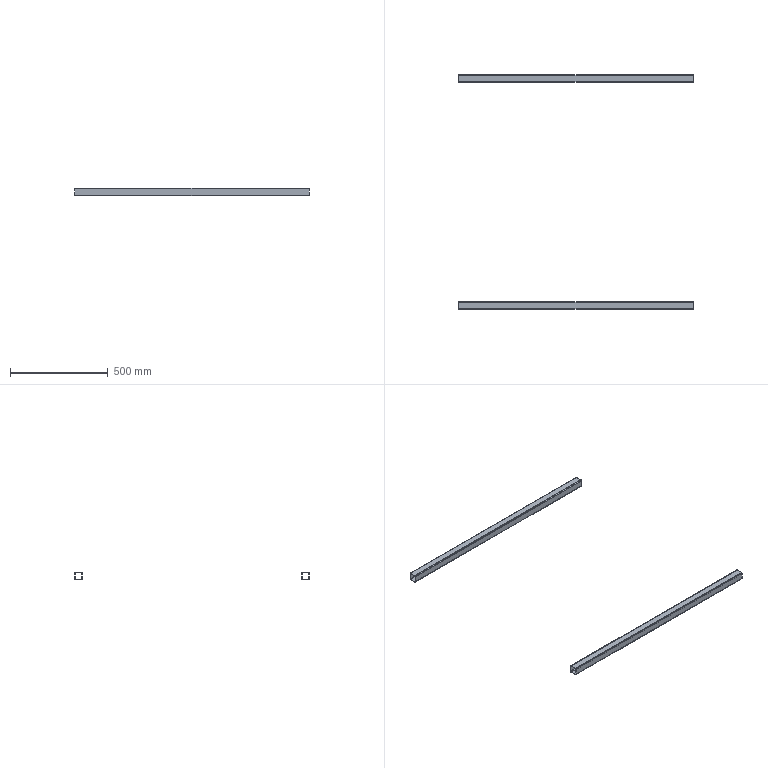Part | SolidWorks | features WeldMemberFeat 1, WeldmentFeature 1 | 2 solids | 36 faces | box 1200 x 1200 x 40 mm | volume 799721 mm3 | plane 20 | cylinder 16 | commonest cylinder face diameters 4.6 x8 9.2 x8
STEP:
#1=CARTESIAN_POINT('',(0.,20.,15.4));
#2=VERTEX_POINT('',#1);
#3=CARTESIAN_POINT('',(0.,15.4,20.));
#4=VERTEX_POINT('',#3);
#5=CARTESIAN_POINT('',(0.,15.4,15.4));
#6=DIRECTION('',(1.,0.,0.));
#7=DIRECTION('',(0.,0.,-1.));
#8=AXIS2_PLACEMENT_3D('',#5,#6,#7);
#9=CIRCLE('',#8,4.6);
#10=EDGE_CURVE('',#2,#4,#9,.T.);
#11=ORIENTED_EDGE('',*,*,#10,.T.);
#12=CARTESIAN_POINT('',(1200.,15.4,20.));
#13=VERTEX_POINT('',#12);
#14=CARTESIAN_POINT('',(1200.,15.4,20.));
#15=DIRECTION('',(-1.,0.,0.));
#16=VECTOR('',#15,1000.);
#17=LINE('',#14,#16);
#18=EDGE_CURVE('',#13,#4,#17,.T.);
#19=ORIENTED_EDGE('',*,*,#18,.F.);
#20=CARTESIAN_POINT('',(1200.,20.,15.4));
#21=VERTEX_POINT('',#20);
#22=CARTESIAN_POINT('',(1200.,15.4,15.4));
#23=DIRECTION('',(1.,0.,0.));
#24=DIRECTION('',(0.,0.,-1.));
#25=AXIS2_PLACEMENT_3D('',#22,#23,#24);
#26=CIRCLE('',#25,4.6);
#27=EDGE_CURVE('',#21,#13,#26,.T.);
#28=ORIENTED_EDGE('',*,*,#27,.F.);
#29=CARTESIAN_POINT('',(1200.,20.,15.4));
#30=DIRECTION('',(-1.,0.,0.));
#31=VECTOR('',#30,1000.);
#32=LINE('',#29,#31);
#33=EDGE_CURVE('',#21,#2,#32,.T.);
#34=ORIENTED_EDGE('',*,*,#33,.T.);
#35=EDGE_LOOP('',(#11,#19,#28,#34));
#36=FACE_OUTER_BOUND('',#35,.T.);
#37=CARTESIAN_POINT('',(1200.,15.4,15.4));
#38=DIRECTION('',(-1.,0.,0.));
#39=DIRECTION('',(0.,0.,1.));
#40=AXIS2_PLACEMENT_3D('',#37,#38,#39);
#41=CYLINDRICAL_SURFACE('',#40,4.6);
#42=ADVANCED_FACE('',(#36),#41,.T.);
#43=CARTESIAN_POINT('',(0.,-15.4,20.));
#44=VERTEX_POINT('',#43);
#45=CARTESIAN_POINT('',(0.,15.4,20.));
#46=DIRECTION('',(0.,-1.,0.));
#47=VECTOR('',#46,1000.);
#48=LINE('',#45,#47);
#49=EDGE_CURVE('',#4,#44,#48,.T.);
#50=ORIENTED_EDGE('',*,*,#49,.T.);
#51=CARTESIAN_POINT('',(1200.,-15.4,20.));
#52=VERTEX_POINT('',#51);
#53=CARTESIAN_POINT('',(1200.,-15.4,20.));
#54=DIRECTION('',(-1.,0.,0.));
#55=VECTOR('',#54,1000.);
#56=LINE('',#53,#55);
#57=EDGE_CURVE('',#52,#44,#56,.T.);
#58=ORIENTED_EDGE('',*,*,#57,.F.);
#59=CARTESIAN_POINT('',(1200.,15.4,20.));
#60=DIRECTION('',(0.,-1.,0.));
#61=VECTOR('',#60,1000.);
#62=LINE('',#59,#61);
#63=EDGE_CURVE('',#13,#52,#62,.T.);
#64=ORIENTED_EDGE('',*,*,#63,.F.);
#65=ORIENTED_EDGE('',*,*,#18,.T.);
#66=EDGE_LOOP('',(#50,#58,#64,#65));
#67=FACE_OUTER_BOUND('',#66,.T.);
#68=CARTESIAN_POINT('',(1200.,15.4,20.));
#69=DIRECTION('',(0.,0.,-1.));
#70=DIRECTION('',(0.,1.,0.));
#71=AXIS2_PLACEMENT_3D('',#68,#69,#70);
#72=PLANE('',#71);
#73=ADVANCED_FACE('',(#67),#72,.F.);
#74=CARTESIAN_POINT('',(0.,-20.,15.4));
#75=VERTEX_POINT('',#74);
#76=CARTESIAN_POINT('',(0.,-15.4,15.4));
#77=DIRECTION('',(1.,0.,0.));
#78=DIRECTION('',(0.,0.,-1.));
#79=AXIS2_PLACEMENT_3D('',#76,#77,#78);
#80=CIRCLE('',#79,4.6);
#81=EDGE_CURVE('',#44,#75,#80,.T.);
#82=ORIENTED_EDGE('',*,*,#81,.T.);
#83=CARTESIAN_POINT('',(1200.,-20.,15.4));
#84=VERTEX_POINT('',#83);
#85=CARTESIAN_POINT('',(1200.,-20.,15.4));
#86=DIRECTION('',(-1.,0.,0.));
#87=VECTOR('',#86,1000.);
#88=LINE('',#85,#87);
#89=EDGE_CURVE('',#84,#75,#88,.T.);
#90=ORIENTED_EDGE('',*,*,#89,.F.);
#91=CARTESIAN_POINT('',(1200.,-15.4,15.4));
#92=DIRECTION('',(1.,0.,0.));
#93=DIRECTION('',(0.,0.,-1.));
#94=AXIS2_PLACEMENT_3D('',#91,#92,#93);
#95=CIRCLE('',#94,4.6);
#96=EDGE_CURVE('',#52,#84,#95,.T.);
#97=ORIENTED_EDGE('',*,*,#96,.F.);
#98=ORIENTED_EDGE('',*,*,#57,.T.);
#99=EDGE_LOOP('',(#82,#90,#97,#98));
#100=FACE_OUTER_BOUND('',#99,.T.);
#101=CARTESIAN_POINT('',(1200.,-15.4,15.4));
#102=DIRECTION('',(-1.,0.,0.));
#103=DIRECTION('',(0.,0.,1.));
#104=AXIS2_PLACEMENT_3D('',#101,#102,#103);
#105=CYLINDRICAL_SURFACE('',#104,4.6);
#106=ADVANCED_FACE('',(#100),#105,.T.);
#107=CARTESIAN_POINT('',(0.,-20.,-15.4));
#108=VERTEX_POINT('',#107);
#109=CARTESIAN_POINT('',(0.,-20.,-15.4));
#110=DIRECTION('',(0.,0.,-1.));
#111=VECTOR('',#110,1000.);
#112=LINE('',#109,#111);
#113=EDGE_CURVE('',#75,#108,#112,.T.);
#114=ORIENTED_EDGE('',*,*,#113,.T.);
#115=CARTESIAN_POINT('',(1200.,-20.,-15.4));
#116=VERTEX_POINT('',#115);
#117=CARTESIAN_POINT('',(1200.,-20.,-15.4));
#118=DIRECTION('',(-1.,0.,0.));
#119=VECTOR('',#118,1000.);
#120=LINE('',#117,#119);
#121=EDGE_CURVE('',#116,#108,#120,.T.);
#122=ORIENTED_EDGE('',*,*,#121,.F.);
#123=CARTESIAN_POINT('',(1200.,-20.,-15.4));
#124=DIRECTION('',(0.,0.,-1.));
#125=VECTOR('',#124,1000.);
#126=LINE('',#123,#125);
#127=EDGE_CURVE('',#84,#116,#126,.T.);
#128=ORIENTED_EDGE('',*,*,#127,.F.);
#129=ORIENTED_EDGE('',*,*,#89,.T.);
#130=EDGE_LOOP('',(#114,#122,#128,#129));
#131=FACE_OUTER_BOUND('',#130,.T.);
#132=CARTESIAN_POINT('',(1200.,-20.,-15.4));
#133=DIRECTION('',(0.,1.,0.));
#134=DIRECTION('',(0.,0.,1.));
#135=AXIS2_PLACEMENT_3D('',#132,#133,#134);
#136=PLANE('',#135);
#137=ADVANCED_FACE('',(#131),#136,.F.);
#138=CARTESIAN_POINT('',(0.,-15.4,-20.));
#139=VERTEX_POINT('',#138);
#140=CARTESIAN_POINT('',(0.,-15.4,-15.4));
#141=DIRECTION('',(1.,0.,0.));
#142=DIRECTION('',(0.,0.,-1.));
#143=AXIS2_PLACEMENT_3D('',#140,#141,#142);
#144=CIRCLE('',#143,4.6);
#145=EDGE_CURVE('',#108,#139,#144,.T.);
#146=ORIENTED_EDGE('',*,*,#145,.T.);
#147=CARTESIAN_POINT('',(1200.,-15.4,-20.));
#148=VERTEX_POINT('',#147);
#149=CARTESIAN_POINT('',(1200.,-15.4,-20.));
#150=DIRECTION('',(-1.,0.,0.));
#151=VECTOR('',#150,1000.);
#152=LINE('',#149,#151);
#153=EDGE_CURVE('',#148,#139,#152,.T.);
#154=ORIENTED_EDGE('',*,*,#153,.F.);
#155=CARTESIAN_POINT('',(1200.,-15.4,-15.4));
#156=DIRECTION('',(1.,0.,0.));
#157=DIRECTION('',(0.,0.,-1.));
#158=AXIS2_PLACEMENT_3D('',#155,#156,#157);
#159=CIRCLE('',#158,4.6);
#160=EDGE_CURVE('',#116,#148,#159,.T.);
#161=ORIENTED_EDGE('',*,*,#160,.F.);
#162=ORIENTED_EDGE('',*,*,#121,.T.);
#163=EDGE_LOOP('',(#146,#154,#161,#162));
#164=FACE_OUTER_BOUND('',#163,.T.);
#165=CARTESIAN_POINT('',(1200.,-15.4,-15.4));
#166=DIRECTION('',(-1.,0.,0.));
#167=DIRECTION('',(0.,0.,1.));
#168=AXIS2_PLACEMENT_3D('',#165,#166,#167);
#169=CYLINDRICAL_SURFACE('',#168,4.6);
#170=ADVANCED_FACE('',(#164),#169,.T.);
#171=CARTESIAN_POINT('',(0.,15.4,-20.));
#172=VERTEX_POINT('',#171);
#173=CARTESIAN_POINT('',(0.,-15.4,-20.));
#174=DIRECTION('',(0.,1.,0.));
#175=VECTOR('',#174,1000.);
#176=LINE('',#173,#175);
#177=EDGE_CURVE('',#139,#172,#176,.T.);
#178=ORIENTED_EDGE('',*,*,#177,.T.);
#179=CARTESIAN_POINT('',(1200.,15.4,-20.));
#180=VERTEX_POINT('',#179);
#181=CARTESIAN_POINT('',(1200.,15.4,-20.));
#182=DIRECTION('',(-1.,0.,0.));
#183=VECTOR('',#182,1000.);
#184=LINE('',#181,#183);
#185=EDGE_CURVE('',#180,#172,#184,.T.);
#186=ORIENTED_EDGE('',*,*,#185,.F.);
#187=CARTESIAN_POINT('',(1200.,-15.4,-20.));
#188=DIRECTION('',(0.,1.,0.));
#189=VECTOR('',#188,1000.);
#190=LINE('',#187,#189);
#191=EDGE_CURVE('',#148,#180,#190,.T.);
#192=ORIENTED_EDGE('',*,*,#191,.F.);
#193=ORIENTED_EDGE('',*,*,#153,.T.);
#194=EDGE_LOOP('',(#178,#186,#192,#193));
#195=FACE_OUTER_BOUND('',#194,.T.);
#196=CARTESIAN_POINT('',(1200.,-15.4,-20.));
#197=DIRECTION('',(0.,0.,1.));
#198=DIRECTION('',(0.,-1.,0.));
#199=AXIS2_PLACEMENT_3D('',#196,#197,#198);
#200=PLANE('',#199);
#201=ADVANCED_FACE('',(#195),#200,.F.);
#202=CARTESIAN_POINT('',(0.,20.,-15.4));
#203=VERTEX_POINT('',#202);
#204=CARTESIAN_POINT('',(0.,15.4,-15.4));
#205=DIRECTION('',(1.,0.,0.));
#206=DIRECTION('',(0.,0.,-1.));
#207=AXIS2_PLACEMENT_3D('',#204,#205,#206);
#208=CIRCLE('',#207,4.6);
#209=EDGE_CURVE('',#172,#203,#208,.T.);
#210=ORIENTED_EDGE('',*,*,#209,.T.);
#211=CARTESIAN_POINT('',(1200.,20.,-15.4));
#212=VERTEX_POINT('',#211);
#213=CARTESIAN_POINT('',(1200.,20.,-15.4));
#214=DIRECTION('',(-1.,0.,0.));
#215=VECTOR('',#214,1000.);
#216=LINE('',#213,#215);
#217=EDGE_CURVE('',#212,#203,#216,.T.);
#218=ORIENTED_EDGE('',*,*,#217,.F.);
#219=CARTESIAN_POINT('',(1200.,15.4,-15.4));
#220=DIRECTION('',(1.,0.,0.));
#221=DIRECTION('',(0.,0.,-1.));
#222=AXIS2_PLACEMENT_3D('',#219,#220,#221);
#223=CIRCLE('',#222,4.6);
#224=EDGE_CURVE('',#180,#212,#223,.T.);
#225=ORIENTED_EDGE('',*,*,#224,.F.);
#226=ORIENTED_EDGE('',*,*,#185,.T.);
#227=EDGE_LOOP('',(#210,#218,#225,#226));
#228=FACE_OUTER_BOUND('',#227,.T.);
#229=CARTESIAN_POINT('',(1200.,15.4,-15.4));
#230=DIRECTION('',(-1.,0.,0.));
#231=DIRECTION('',(0.,0.,1.));
#232=AXIS2_PLACEMENT_3D('',#229,#230,#231);
#233=CYLINDRICAL_SURFACE('',#232,4.6);
#234=ADVANCED_FACE('',(#228),#233,.T.);
#235=CARTESIAN_POINT('',(0.,-15.4,17.7));
#236=VERTEX_POINT('',#235);
#237=CARTESIAN_POINT('',(0.,-17.7,15.4));
#238=VERTEX_POINT('',#237);
#239=CARTESIAN_POINT('',(0.,-15.4,15.4));
#240=DIRECTION('',(1.,0.,0.));
#241=DIRECTION('',(0.,0.,-1.));
#242=AXIS2_PLACEMENT_3D('',#239,#240,#241);
#243=CIRCLE('',#242,2.3);
#244=EDGE_CURVE('',#236,#238,#243,.T.);
#245=ORIENTED_EDGE('',*,*,#244,.F.);
#246=CARTESIAN_POINT('',(1200.,-15.4,17.7));
#247=VERTEX_POINT('',#246);
#248=CARTESIAN_POINT('',(1200.,-15.4,17.7));
#249=DIRECTION('',(-1.,0.,0.));
#250=VECTOR('',#249,1000.);
#251=LINE('',#248,#250);
#252=EDGE_CURVE('',#247,#236,#251,.T.);
#253=ORIENTED_EDGE('',*,*,#252,.F.);
#254=CARTESIAN_POINT('',(1200.,-17.7,15.4));
#255=VERTEX_POINT('',#254);
#256=CARTESIAN_POINT('',(1200.,-15.4,15.4));
#257=DIRECTION('',(1.,0.,0.));
#258=DIRECTION('',(0.,0.,-1.));
#259=AXIS2_PLACEMENT_3D('',#256,#257,#258);
#260=CIRCLE('',#259,2.3);
#261=EDGE_CURVE('',#247,#255,#260,.T.);
#262=ORIENTED_EDGE('',*,*,#261,.T.);
#263=CARTESIAN_POINT('',(1200.,-17.7,15.4));
#264=DIRECTION('',(-1.,0.,0.));
#265=VECTOR('',#264,1000.);
#266=LINE('',#263,#265);
#267=EDGE_CURVE('',#255,#238,#266,.T.);
#268=ORIENTED_EDGE('',*,*,#267,.T.);
#269=EDGE_LOOP('',(#245,#253,#262,#268));
#270=FACE_OUTER_BOUND('',#269,.T.);
#271=CARTESIAN_POINT('',(1200.,-15.4,15.4));
#272=DIRECTION('',(-1.,0.,0.));
#273=DIRECTION('',(0.,0.,1.));
#274=AXIS2_PLACEMENT_3D('',#271,#272,#273);
#275=CYLINDRICAL_SURFACE('',#274,2.3);
#276=ADVANCED_FACE('',(#270),#275,.F.);
#277=CARTESIAN_POINT('',(0.,15.4,17.7));
#278=VERTEX_POINT('',#277);
#279=CARTESIAN_POINT('',(0.,15.4,17.7));
#280=DIRECTION('',(0.,-1.,0.));
#281=VECTOR('',#280,1000.);
#282=LINE('',#279,#281);
#283=EDGE_CURVE('',#278,#236,#282,.T.);
#284=ORIENTED_EDGE('',*,*,#283,.F.);
#285=CARTESIAN_POINT('',(1200.,15.4,17.7));
#286=VERTEX_POINT('',#285);
#287=CARTESIAN_POINT('',(1200.,15.4,17.7));
#288=DIRECTION('',(-1.,0.,0.));
#289=VECTOR('',#288,1000.);
#290=LINE('',#287,#289);
#291=EDGE_CURVE('',#286,#278,#290,.T.);
#292=ORIENTED_EDGE('',*,*,#291,.F.);
#293=CARTESIAN_POINT('',(1200.,15.4,17.7));
#294=DIRECTION('',(0.,-1.,0.));
#295=VECTOR('',#294,1000.);
#296=LINE('',#293,#295);
#297=EDGE_CURVE('',#286,#247,#296,.T.);
#298=ORIENTED_EDGE('',*,*,#297,.T.);
#299=ORIENTED_EDGE('',*,*,#252,.T.);
#300=EDGE_LOOP('',(#284,#292,#298,#299));
#301=FACE_OUTER_BOUND('',#300,.T.);
#302=CARTESIAN_POINT('',(1200.,15.4,17.7));
#303=DIRECTION('',(0.,0.,-1.));
#304=DIRECTION('',(0.,1.,0.));
#305=AXIS2_PLACEMENT_3D('',#302,#303,#304);
#306=PLANE('',#305);
#307=ADVANCED_FACE('',(#301),#306,.T.);
#308=CARTESIAN_POINT('',(0.,17.7,15.4));
#309=VERTEX_POINT('',#308);
#310=CARTESIAN_POINT('',(0.,15.4,15.4));
#311=DIRECTION('',(1.,0.,0.));
#312=DIRECTION('',(0.,0.,-1.));
#313=AXIS2_PLACEMENT_3D('',#310,#311,#312);
#314=CIRCLE('',#313,2.3);
#315=EDGE_CURVE('',#309,#278,#314,.T.);
#316=ORIENTED_EDGE('',*,*,#315,.F.);
#317=CARTESIAN_POINT('',(1200.,17.7,15.4));
#318=VERTEX_POINT('',#317);
#319=CARTESIAN_POINT('',(1200.,17.7,15.4));
#320=DIRECTION('',(-1.,0.,0.));
#321=VECTOR('',#320,1000.);
#322=LINE('',#319,#321);
#323=EDGE_CURVE('',#318,#309,#322,.T.);
#324=ORIENTED_EDGE('',*,*,#323,.F.);
#325=CARTESIAN_POINT('',(1200.,15.4,15.4));
#326=DIRECTION('',(1.,0.,0.));
#327=DIRECTION('',(0.,0.,-1.));
#328=AXIS2_PLACEMENT_3D('',#325,#326,#327);
#329=CIRCLE('',#328,2.3);
#330=EDGE_CURVE('',#318,#286,#329,.T.);
#331=ORIENTED_EDGE('',*,*,#330,.T.);
#332=ORIENTED_EDGE('',*,*,#291,.T.);
#333=EDGE_LOOP('',(#316,#324,#331,#332));
#334=FACE_OUTER_BOUND('',#333,.T.);
#335=CARTESIAN_POINT('',(1200.,15.4,15.4));
#336=DIRECTION('',(-1.,0.,0.));
#337=DIRECTION('',(0.,0.,1.));
#338=AXIS2_PLACEMENT_3D('',#335,#336,#337);
#339=CYLINDRICAL_SURFACE('',#338,2.3);
#340=ADVANCED_FACE('',(#334),#339,.F.);
#341=CARTESIAN_POINT('',(0.,17.7,-15.4));
#342=VERTEX_POINT('',#341);
#343=CARTESIAN_POINT('',(0.,17.7,15.4));
#344=DIRECTION('',(0.,0.,1.));
#345=VECTOR('',#344,1000.);
#346=LINE('',#343,#345);
#347=EDGE_CURVE('',#342,#309,#346,.T.);
#348=ORIENTED_EDGE('',*,*,#347,.F.);
#349=CARTESIAN_POINT('',(1200.,17.7,-15.4));
#350=VERTEX_POINT('',#349);
#351=CARTESIAN_POINT('',(1200.,17.7,-15.4));
#352=DIRECTION('',(-1.,0.,0.));
#353=VECTOR('',#352,1000.);
#354=LINE('',#351,#353);
#355=EDGE_CURVE('',#350,#342,#354,.T.);
#356=ORIENTED_EDGE('',*,*,#355,.F.);
#357=CARTESIAN_POINT('',(1200.,17.7,15.4));
#358=DIRECTION('',(0.,0.,1.));
#359=VECTOR('',#358,1000.);
#360=LINE('',#357,#359);
#361=EDGE_CURVE('',#350,#318,#360,.T.);
#362=ORIENTED_EDGE('',*,*,#361,.T.);
#363=ORIENTED_EDGE('',*,*,#323,.T.);
#364=EDGE_LOOP('',(#348,#356,#362,#363));
#365=FACE_OUTER_BOUND('',#364,.T.);
#366=CARTESIAN_POINT('',(1200.,17.7,15.4));
#367=DIRECTION('',(0.,-1.,0.));
#368=DIRECTION('',(0.,0.,-1.));
#369=AXIS2_PLACEMENT_3D('',#366,#367,#368);
#370=PLANE('',#369);
#371=ADVANCED_FACE('',(#365),#370,.T.);
#372=CARTESIAN_POINT('',(0.,15.4,-17.7));
#373=VERTEX_POINT('',#372);
#374=CARTESIAN_POINT('',(0.,15.4,-15.4));
#375=DIRECTION('',(1.,0.,0.));
#376=DIRECTION('',(0.,0.,-1.));
#377=AXIS2_PLACEMENT_3D('',#374,#375,#376);
#378=CIRCLE('',#377,2.3);
#379=EDGE_CURVE('',#373,#342,#378,.T.);
#380=ORIENTED_EDGE('',*,*,#379,.F.);
#381=CARTESIAN_POINT('',(1200.,15.4,-17.7));
#382=VERTEX_POINT('',#381);
#383=CARTESIAN_POINT('',(1200.,15.4,-17.7));
#384=DIRECTION('',(-1.,0.,0.));
#385=VECTOR('',#384,1000.);
#386=LINE('',#383,#385);
#387=EDGE_CURVE('',#382,#373,#386,.T.);
#388=ORIENTED_EDGE('',*,*,#387,.F.);
#389=CARTESIAN_POINT('',(1200.,15.4,-15.4));
#390=DIRECTION('',(1.,0.,0.));
#391=DIRECTION('',(0.,0.,-1.));
#392=AXIS2_PLACEMENT_3D('',#389,#390,#391);
#393=CIRCLE('',#392,2.3);
#394=EDGE_CURVE('',#382,#350,#393,.T.);
#395=ORIENTED_EDGE('',*,*,#394,.T.);
#396=ORIENTED_EDGE('',*,*,#355,.T.);
#397=EDGE_LOOP('',(#380,#388,#395,#396));
#398=FACE_OUTER_BOUND('',#397,.T.);
#399=CARTESIAN_POINT('',(1200.,15.4,-15.4));
#400=DIRECTION('',(-1.,0.,0.));
#401=DIRECTION('',(0.,0.,1.));
#402=AXIS2_PLACEMENT_3D('',#399,#400,#401);
#403=CYLINDRICAL_SURFACE('',#402,2.3);
#404=ADVANCED_FACE('',(#398),#403,.F.);
#405=CARTESIAN_POINT('',(0.,-15.4,-17.7));
#406=VERTEX_POINT('',#405);
#407=CARTESIAN_POINT('',(0.,-15.4,-17.7));
#408=DIRECTION('',(0.,1.,0.));
#409=VECTOR('',#408,1000.);
#410=LINE('',#407,#409);
#411=EDGE_CURVE('',#406,#373,#410,.T.);
#412=ORIENTED_EDGE('',*,*,#411,.F.);
#413=CARTESIAN_POINT('',(1200.,-15.4,-17.7));
#414=VERTEX_POINT('',#413);
#415=CARTESIAN_POINT('',(1200.,-15.4,-17.7));
#416=DIRECTION('',(-1.,0.,0.));
#417=VECTOR('',#416,1000.);
#418=LINE('',#415,#417);
#419=EDGE_CURVE('',#414,#406,#418,.T.);
#420=ORIENTED_EDGE('',*,*,#419,.F.);
#421=CARTESIAN_POINT('',(1200.,-15.4,-17.7));
#422=DIRECTION('',(0.,1.,0.));
#423=VECTOR('',#422,1000.);
#424=LINE('',#421,#423);
#425=EDGE_CURVE('',#414,#382,#424,.T.);
#426=ORIENTED_EDGE('',*,*,#425,.T.);
#427=ORIENTED_EDGE('',*,*,#387,.T.);
#428=EDGE_LOOP('',(#412,#420,#426,#427));
#429=FACE_OUTER_BOUND('',#428,.T.);
#430=CARTESIAN_POINT('',(1200.,-15.4,-17.7));
#431=DIRECTION('',(0.,0.,1.));
#432=DIRECTION('',(0.,-1.,0.));
#433=AXIS2_PLACEMENT_3D('',#430,#431,#432);
#434=PLANE('',#433);
#435=ADVANCED_FACE('',(#429),#434,.T.);
#436=CARTESIAN_POINT('',(0.,-17.7,-15.4));
#437=VERTEX_POINT('',#436);
#438=CARTESIAN_POINT('',(0.,-15.4,-15.4));
#439=DIRECTION('',(1.,0.,0.));
#440=DIRECTION('',(0.,0.,-1.));
#441=AXIS2_PLACEMENT_3D('',#438,#439,#440);
#442=CIRCLE('',#441,2.3);
#443=EDGE_CURVE('',#437,#406,#442,.T.);
#444=ORIENTED_EDGE('',*,*,#443,.F.);
#445=CARTESIAN_POINT('',(1200.,-17.7,-15.4));
#446=VERTEX_POINT('',#445);
#447=CARTESIAN_POINT('',(1200.,-17.7,-15.4));
#448=DIRECTION('',(-1.,0.,0.));
#449=VECTOR('',#448,1000.);
#450=LINE('',#447,#449);
#451=EDGE_CURVE('',#446,#437,#450,.T.);
#452=ORIENTED_EDGE('',*,*,#451,.F.);
#453=CARTESIAN_POINT('',(1200.,-15.4,-15.4));
#454=DIRECTION('',(1.,0.,0.));
#455=DIRECTION('',(0.,0.,-1.));
#456=AXIS2_PLACEMENT_3D('',#453,#454,#455);
#457=CIRCLE('',#456,2.3);
#458=EDGE_CURVE('',#446,#414,#457,.T.);
#459=ORIENTED_EDGE('',*,*,#458,.T.);
#460=ORIENTED_EDGE('',*,*,#419,.T.);
#461=EDGE_LOOP('',(#444,#452,#459,#460));
#462=FACE_OUTER_BOUND('',#461,.T.);
#463=CARTESIAN_POINT('',(1200.,-15.4,-15.4));
#464=DIRECTION('',(-1.,0.,0.));
#465=DIRECTION('',(0.,0.,1.));
#466=AXIS2_PLACEMENT_3D('',#463,#464,#465);
#467=CYLINDRICAL_SURFACE('',#466,2.3);
#468=ADVANCED_FACE('',(#462),#467,.F.);
#469=CARTESIAN_POINT('',(0.,-17.7,-15.4));
#470=DIRECTION('',(0.,0.,-1.));
#471=VECTOR('',#470,1000.);
#472=LINE('',#469,#471);
#473=EDGE_CURVE('',#238,#437,#472,.T.);
#474=ORIENTED_EDGE('',*,*,#473,.F.);
#475=ORIENTED_EDGE('',*,*,#267,.F.);
#476=CARTESIAN_POINT('',(1200.,-17.7,-15.4));
#477=DIRECTION('',(0.,0.,-1.));
#478=VECTOR('',#477,1000.);
#479=LINE('',#476,#478);
#480=EDGE_CURVE('',#255,#446,#479,.T.);
#481=ORIENTED_EDGE('',*,*,#480,.T.);
#482=ORIENTED_EDGE('',*,*,#451,.T.);
#483=EDGE_LOOP('',(#474,#475,#481,#482));
#484=FACE_OUTER_BOUND('',#483,.T.);
#485=CARTESIAN_POINT('',(1200.,-17.7,-15.4));
#486=DIRECTION('',(0.,1.,0.));
#487=DIRECTION('',(0.,0.,1.));
#488=AXIS2_PLACEMENT_3D('',#485,#486,#487);
#489=PLANE('',#488);
#490=ADVANCED_FACE('',(#484),#489,.T.);
#491=CARTESIAN_POINT('',(0.,20.,15.4));
#492=DIRECTION('',(0.,0.,1.));
#493=VECTOR('',#492,1000.);
#494=LINE('',#491,#493);
#495=EDGE_CURVE('',#203,#2,#494,.T.);
#496=ORIENTED_EDGE('',*,*,#495,.T.);
#497=ORIENTED_EDGE('',*,*,#33,.F.);
#498=CARTESIAN_POINT('',(1200.,20.,15.4));
#499=DIRECTION('',(0.,0.,1.));
#500=VECTOR('',#499,1000.);
#501=LINE('',#498,#500);
#502=EDGE_CURVE('',#212,#21,#501,.T.);
#503=ORIENTED_EDGE('',*,*,#502,.F.);
#504=ORIENTED_EDGE('',*,*,#217,.T.);
#505=EDGE_LOOP('',(#496,#497,#503,#504));
#506=FACE_OUTER_BOUND('',#505,.T.);
#507=CARTESIAN_POINT('',(1200.,20.,15.4));
#508=DIRECTION('',(0.,-1.,0.));
#509=DIRECTION('',(0.,0.,-1.));
#510=AXIS2_PLACEMENT_3D('',#507,#508,#509);
#511=PLANE('',#510);
#512=ADVANCED_FACE('',(#506),#511,.F.);
#513=ORIENTED_EDGE('',*,*,#261,.F.);
#514=ORIENTED_EDGE('',*,*,#297,.F.);
#515=ORIENTED_EDGE('',*,*,#330,.F.);
#516=ORIENTED_EDGE('',*,*,#361,.F.);
#517=ORIENTED_EDGE('',*,*,#394,.F.);
#518=ORIENTED_EDGE('',*,*,#425,.F.);
#519=ORIENTED_EDGE('',*,*,#458,.F.);
#520=ORIENTED_EDGE('',*,*,#480,.F.);
#521=EDGE_LOOP('',(#513,#514,#515,#516,#517,#518,#519,#520));
#522=FACE_BOUND('',#521,.T.);
#523=ORIENTED_EDGE('',*,*,#27,.T.);
#524=ORIENTED_EDGE('',*,*,#63,.T.);
#525=ORIENTED_EDGE('',*,*,#96,.T.);
#526=ORIENTED_EDGE('',*,*,#127,.T.);
#527=ORIENTED_EDGE('',*,*,#160,.T.);
#528=ORIENTED_EDGE('',*,*,#191,.T.);
#529=ORIENTED_EDGE('',*,*,#224,.T.);
#530=ORIENTED_EDGE('',*,*,#502,.T.);
#531=EDGE_LOOP('',(#523,#524,#525,#526,#527,#528,#529,#530));
#532=FACE_OUTER_BOUND('',#531,.T.);
#533=CARTESIAN_POINT('',(1200.,15.4,15.4));
#534=DIRECTION('',(1.,0.,0.));
#535=DIRECTION('',(0.,0.,-1.));
#536=AXIS2_PLACEMENT_3D('',#533,#534,#535);
#537=PLANE('',#536);
#538=ADVANCED_FACE('',(#522,#532),#537,.T.);
#539=ORIENTED_EDGE('',*,*,#244,.T.);
#540=ORIENTED_EDGE('',*,*,#473,.T.);
#541=ORIENTED_EDGE('',*,*,#443,.T.);
#542=ORIENTED_EDGE('',*,*,#411,.T.);
#543=ORIENTED_EDGE('',*,*,#379,.T.);
#544=ORIENTED_EDGE('',*,*,#347,.T.);
#545=ORIENTED_EDGE('',*,*,#315,.T.);
#546=ORIENTED_EDGE('',*,*,#283,.T.);
#547=EDGE_LOOP('',(#539,#540,#541,#542,#543,#544,#545,#546));
#548=FACE_BOUND('',#547,.T.);
#549=ORIENTED_EDGE('',*,*,#10,.F.);
#550=ORIENTED_EDGE('',*,*,#495,.F.);
#551=ORIENTED_EDGE('',*,*,#209,.F.);
#552=ORIENTED_EDGE('',*,*,#177,.F.);
#553=ORIENTED_EDGE('',*,*,#145,.F.);
#554=ORIENTED_EDGE('',*,*,#113,.F.);
#555=ORIENTED_EDGE('',*,*,#81,.F.);
#556=ORIENTED_EDGE('',*,*,#49,.F.);
#557=EDGE_LOOP('',(#549,#550,#551,#552,#553,#554,#555,#556));
#558=FACE_OUTER_BOUND('',#557,.T.);
#559=CARTESIAN_POINT('',(0.,15.4,15.4));
#560=DIRECTION('',(1.,0.,0.));
#561=DIRECTION('',(0.,0.,-1.));
#562=AXIS2_PLACEMENT_3D('',#559,#560,#561);
#563=PLANE('',#562);
#564=ADVANCED_FACE('',(#548,#558),#563,.F.);
#565=CLOSED_SHELL('',(#42,#73,#106,#137,#170,#201,#234,#276,#307,#340,#371,#404,#435,#468,#490,#512,#538,#564));
#566=MANIFOLD_SOLID_BREP('',#565);
#567=CARTESIAN_POINT('',(0.,1180.,15.4));
#568=VERTEX_POINT('',#567);
#569=CARTESIAN_POINT('',(0.,1175.4,20.));
#570=VERTEX_POINT('',#569);
#571=CARTESIAN_POINT('',(0.,1175.4,15.4));
#572=DIRECTION('',(1.,0.,0.));
#573=DIRECTION('',(0.,0.,-1.));
#574=AXIS2_PLACEMENT_3D('',#571,#572,#573);
#575=CIRCLE('',#574,4.6);
#576=EDGE_CURVE('',#568,#570,#575,.T.);
#577=ORIENTED_EDGE('',*,*,#576,.T.);
#578=CARTESIAN_POINT('',(1200.,1175.4,20.));
#579=VERTEX_POINT('',#578);
#580=CARTESIAN_POINT('',(1200.,1175.4,20.));
#581=DIRECTION('',(-1.,0.,0.));
#582=VECTOR('',#581,1000.);
#583=LINE('',#580,#582);
#584=EDGE_CURVE('',#579,#570,#583,.T.);
#585=ORIENTED_EDGE('',*,*,#584,.F.);
#586=CARTESIAN_POINT('',(1200.,1180.,15.4));
#587=VERTEX_POINT('',#586);
#588=CARTESIAN_POINT('',(1200.,1175.4,15.4));
#589=DIRECTION('',(1.,0.,0.));
#590=DIRECTION('',(0.,0.,-1.));
#591=AXIS2_PLACEMENT_3D('',#588,#589,#590);
#592=CIRCLE('',#591,4.6);
#593=EDGE_CURVE('',#587,#579,#592,.T.);
#594=ORIENTED_EDGE('',*,*,#593,.F.);
#595=CARTESIAN_POINT('',(1200.,1180.,15.4));
#596=DIRECTION('',(-1.,0.,0.));
#597=VECTOR('',#596,1000.);
#598=LINE('',#595,#597);
#599=EDGE_CURVE('',#587,#568,#598,.T.);
#600=ORIENTED_EDGE('',*,*,#599,.T.);
#601=EDGE_LOOP('',(#577,#585,#594,#600));
#602=FACE_OUTER_BOUND('',#601,.T.);
#603=CARTESIAN_POINT('',(1200.,1175.4,15.4));
#604=DIRECTION('',(-1.,0.,0.));
#605=DIRECTION('',(0.,0.,1.));
#606=AXIS2_PLACEMENT_3D('',#603,#604,#605);
#607=CYLINDRICAL_SURFACE('',#606,4.6);
#608=ADVANCED_FACE('',(#602),#607,.T.);
#609=CARTESIAN_POINT('',(0.,1144.6,20.));
#610=VERTEX_POINT('',#609);
#611=CARTESIAN_POINT('',(0.,1175.4,20.));
#612=DIRECTION('',(0.,-1.,0.));
#613=VECTOR('',#612,1000.);
#614=LINE('',#611,#613);
#615=EDGE_CURVE('',#570,#610,#614,.T.);
#616=ORIENTED_EDGE('',*,*,#615,.T.);
#617=CARTESIAN_POINT('',(1200.,1144.6,20.));
#618=VERTEX_POINT('',#617);
#619=CARTESIAN_POINT('',(1200.,1144.6,20.));
#620=DIRECTION('',(-1.,0.,0.));
#621=VECTOR('',#620,1000.);
#622=LINE('',#619,#621);
#623=EDGE_CURVE('',#618,#610,#622,.T.);
#624=ORIENTED_EDGE('',*,*,#623,.F.);
#625=CARTESIAN_POINT('',(1200.,1175.4,20.));
#626=DIRECTION('',(0.,-1.,0.));
#627=VECTOR('',#626,1000.);
#628=LINE('',#625,#627);
#629=EDGE_CURVE('',#579,#618,#628,.T.);
#630=ORIENTED_EDGE('',*,*,#629,.F.);
#631=ORIENTED_EDGE('',*,*,#584,.T.);
#632=EDGE_LOOP('',(#616,#624,#630,#631));
#633=FACE_OUTER_BOUND('',#632,.T.);
#634=CARTESIAN_POINT('',(1200.,1175.4,20.));
#635=DIRECTION('',(0.,0.,-1.));
#636=DIRECTION('',(0.,1.,0.));
#637=AXIS2_PLACEMENT_3D('',#634,#635,#636);
#638=PLANE('',#637);
#639=ADVANCED_FACE('',(#633),#638,.F.);
#640=CARTESIAN_POINT('',(0.,1140.,15.4));
#641=VERTEX_POINT('',#640);
#642=CARTESIAN_POINT('',(0.,1144.6,15.4));
#643=DIRECTION('',(1.,0.,0.));
#644=DIRECTION('',(0.,0.,-1.));
#645=AXIS2_PLACEMENT_3D('',#642,#643,#644);
#646=CIRCLE('',#645,4.6);
#647=EDGE_CURVE('',#610,#641,#646,.T.);
#648=ORIENTED_EDGE('',*,*,#647,.T.);
#649=CARTESIAN_POINT('',(1200.,1140.,15.4));
#650=VERTEX_POINT('',#649);
#651=CARTESIAN_POINT('',(1200.,1140.,15.4));
#652=DIRECTION('',(-1.,0.,0.));
#653=VECTOR('',#652,1000.);
#654=LINE('',#651,#653);
#655=EDGE_CURVE('',#650,#641,#654,.T.);
#656=ORIENTED_EDGE('',*,*,#655,.F.);
#657=CARTESIAN_POINT('',(1200.,1144.6,15.4));
#658=DIRECTION('',(1.,0.,0.));
#659=DIRECTION('',(0.,0.,-1.));
#660=AXIS2_PLACEMENT_3D('',#657,#658,#659);
#661=CIRCLE('',#660,4.6);
#662=EDGE_CURVE('',#618,#650,#661,.T.);
#663=ORIENTED_EDGE('',*,*,#662,.F.);
#664=ORIENTED_EDGE('',*,*,#623,.T.);
#665=EDGE_LOOP('',(#648,#656,#663,#664));
#666=FACE_OUTER_BOUND('',#665,.T.);
#667=CARTESIAN_POINT('',(1200.,1144.6,15.4));
#668=DIRECTION('',(-1.,0.,0.));
#669=DIRECTION('',(0.,0.,1.));
#670=AXIS2_PLACEMENT_3D('',#667,#668,#669);
#671=CYLINDRICAL_SURFACE('',#670,4.6);
#672=ADVANCED_FACE('',(#666),#671,.T.);
#673=CARTESIAN_POINT('',(0.,1140.,-15.4));
#674=VERTEX_POINT('',#673);
#675=CARTESIAN_POINT('',(0.,1140.,-15.4));
#676=DIRECTION('',(0.,0.,-1.));
#677=VECTOR('',#676,1000.);
#678=LINE('',#675,#677);
#679=EDGE_CURVE('',#641,#674,#678,.T.);
#680=ORIENTED_EDGE('',*,*,#679,.T.);
#681=CARTESIAN_POINT('',(1200.,1140.,-15.4));
#682=VERTEX_POINT('',#681);
#683=CARTESIAN_POINT('',(1200.,1140.,-15.4));
#684=DIRECTION('',(-1.,0.,0.));
#685=VECTOR('',#684,1000.);
#686=LINE('',#683,#685);
#687=EDGE_CURVE('',#682,#674,#686,.T.);
#688=ORIENTED_EDGE('',*,*,#687,.F.);
#689=CARTESIAN_POINT('',(1200.,1140.,-15.4));
#690=DIRECTION('',(0.,0.,-1.));
#691=VECTOR('',#690,1000.);
#692=LINE('',#689,#691);
#693=EDGE_CURVE('',#650,#682,#692,.T.);
#694=ORIENTED_EDGE('',*,*,#693,.F.);
#695=ORIENTED_EDGE('',*,*,#655,.T.);
#696=EDGE_LOOP('',(#680,#688,#694,#695));
#697=FACE_OUTER_BOUND('',#696,.T.);
#698=CARTESIAN_POINT('',(1200.,1140.,-15.4));
#699=DIRECTION('',(0.,1.,0.));
#700=DIRECTION('',(0.,0.,1.));
#701=AXIS2_PLACEMENT_3D('',#698,#699,#700);
#702=PLANE('',#701);
#703=ADVANCED_FACE('',(#697),#702,.F.);
#704=CARTESIAN_POINT('',(0.,1144.6,-20.));
#705=VERTEX_POINT('',#704);
#706=CARTESIAN_POINT('',(0.,1144.6,-15.4));
#707=DIRECTION('',(1.,0.,0.));
#708=DIRECTION('',(0.,0.,-1.));
#709=AXIS2_PLACEMENT_3D('',#706,#707,#708);
#710=CIRCLE('',#709,4.6);
#711=EDGE_CURVE('',#674,#705,#710,.T.);
#712=ORIENTED_EDGE('',*,*,#711,.T.);
#713=CARTESIAN_POINT('',(1200.,1144.6,-20.));
#714=VERTEX_POINT('',#713);
#715=CARTESIAN_POINT('',(1200.,1144.6,-20.));
#716=DIRECTION('',(-1.,0.,0.));
#717=VECTOR('',#716,1000.);
#718=LINE('',#715,#717);
#719=EDGE_CURVE('',#714,#705,#718,.T.);
#720=ORIENTED_EDGE('',*,*,#719,.F.);
#721=CARTESIAN_POINT('',(1200.,1144.6,-15.4));
#722=DIRECTION('',(1.,0.,0.));
#723=DIRECTION('',(0.,0.,-1.));
#724=AXIS2_PLACEMENT_3D('',#721,#722,#723);
#725=CIRCLE('',#724,4.6);
#726=EDGE_CURVE('',#682,#714,#725,.T.);
#727=ORIENTED_EDGE('',*,*,#726,.F.);
#728=ORIENTED_EDGE('',*,*,#687,.T.);
#729=EDGE_LOOP('',(#712,#720,#727,#728));
#730=FACE_OUTER_BOUND('',#729,.T.);
#731=CARTESIAN_POINT('',(1200.,1144.6,-15.4));
#732=DIRECTION('',(-1.,0.,0.));
#733=DIRECTION('',(0.,0.,1.));
#734=AXIS2_PLACEMENT_3D('',#731,#732,#733);
#735=CYLINDRICAL_SURFACE('',#734,4.6);
#736=ADVANCED_FACE('',(#730),#735,.T.);
#737=CARTESIAN_POINT('',(0.,1175.4,-20.));
#738=VERTEX_POINT('',#737);
#739=CARTESIAN_POINT('',(0.,1144.6,-20.));
#740=DIRECTION('',(0.,1.,0.));
#741=VECTOR('',#740,1000.);
#742=LINE('',#739,#741);
#743=EDGE_CURVE('',#705,#738,#742,.T.);
#744=ORIENTED_EDGE('',*,*,#743,.T.);
#745=CARTESIAN_POINT('',(1200.,1175.4,-20.));
#746=VERTEX_POINT('',#745);
#747=CARTESIAN_POINT('',(1200.,1175.4,-20.));
#748=DIRECTION('',(-1.,0.,0.));
#749=VECTOR('',#748,1000.);
#750=LINE('',#747,#749);
#751=EDGE_CURVE('',#746,#738,#750,.T.);
#752=ORIENTED_EDGE('',*,*,#751,.F.);
#753=CARTESIAN_POINT('',(1200.,1144.6,-20.));
#754=DIRECTION('',(0.,1.,0.));
#755=VECTOR('',#754,1000.);
#756=LINE('',#753,#755);
#757=EDGE_CURVE('',#714,#746,#756,.T.);
#758=ORIENTED_EDGE('',*,*,#757,.F.);
#759=ORIENTED_EDGE('',*,*,#719,.T.);
#760=EDGE_LOOP('',(#744,#752,#758,#759));
#761=FACE_OUTER_BOUND('',#760,.T.);
#762=CARTESIAN_POINT('',(1200.,1144.6,-20.));
#763=DIRECTION('',(0.,0.,1.));
#764=DIRECTION('',(0.,-1.,0.));
#765=AXIS2_PLACEMENT_3D('',#762,#763,#764);
#766=PLANE('',#765);
#767=ADVANCED_FACE('',(#761),#766,.F.);
#768=CARTESIAN_POINT('',(0.,1180.,-15.4));
#769=VERTEX_POINT('',#768);
#770=CARTESIAN_POINT('',(0.,1175.4,-15.4));
#771=DIRECTION('',(1.,0.,0.));
#772=DIRECTION('',(0.,0.,-1.));
#773=AXIS2_PLACEMENT_3D('',#770,#771,#772);
#774=CIRCLE('',#773,4.6);
#775=EDGE_CURVE('',#738,#769,#774,.T.);
#776=ORIENTED_EDGE('',*,*,#775,.T.);
#777=CARTESIAN_POINT('',(1200.,1180.,-15.4));
#778=VERTEX_POINT('',#777);
#779=CARTESIAN_POINT('',(1200.,1180.,-15.4));
#780=DIRECTION('',(-1.,0.,0.));
#781=VECTOR('',#780,1000.);
#782=LINE('',#779,#781);
#783=EDGE_CURVE('',#778,#769,#782,.T.);
#784=ORIENTED_EDGE('',*,*,#783,.F.);
#785=CARTESIAN_POINT('',(1200.,1175.4,-15.4));
#786=DIRECTION('',(1.,0.,0.));
#787=DIRECTION('',(0.,0.,-1.));
#788=AXIS2_PLACEMENT_3D('',#785,#786,#787);
#789=CIRCLE('',#788,4.6);
#790=EDGE_CURVE('',#746,#778,#789,.T.);
#791=ORIENTED_EDGE('',*,*,#790,.F.);
#792=ORIENTED_EDGE('',*,*,#751,.T.);
#793=EDGE_LOOP('',(#776,#784,#791,#792));
#794=FACE_OUTER_BOUND('',#793,.T.);
#795=CARTESIAN_POINT('',(1200.,1175.4,-15.4));
#796=DIRECTION('',(-1.,0.,0.));
#797=DIRECTION('',(0.,0.,1.));
#798=AXIS2_PLACEMENT_3D('',#795,#796,#797);
#799=CYLINDRICAL_SURFACE('',#798,4.6);
#800=ADVANCED_FACE('',(#794),#799,.T.);
#801=CARTESIAN_POINT('',(0.,1144.6,17.7));
#802=VERTEX_POINT('',#801);
#803=CARTESIAN_POINT('',(0.,1142.3,15.4));
#804=VERTEX_POINT('',#803);
#805=CARTESIAN_POINT('',(0.,1144.6,15.4));
#806=DIRECTION('',(1.,0.,0.));
#807=DIRECTION('',(0.,0.,-1.));
#808=AXIS2_PLACEMENT_3D('',#805,#806,#807);
#809=CIRCLE('',#808,2.3);
#810=EDGE_CURVE('',#802,#804,#809,.T.);
#811=ORIENTED_EDGE('',*,*,#810,.F.);
#812=CARTESIAN_POINT('',(1200.,1144.6,17.7));
#813=VERTEX_POINT('',#812);
#814=CARTESIAN_POINT('',(1200.,1144.6,17.7));
#815=DIRECTION('',(-1.,0.,0.));
#816=VECTOR('',#815,1000.);
#817=LINE('',#814,#816);
#818=EDGE_CURVE('',#813,#802,#817,.T.);
#819=ORIENTED_EDGE('',*,*,#818,.F.);
#820=CARTESIAN_POINT('',(1200.,1142.3,15.4));
#821=VERTEX_POINT('',#820);
#822=CARTESIAN_POINT('',(1200.,1144.6,15.4));
#823=DIRECTION('',(1.,0.,0.));
#824=DIRECTION('',(0.,0.,-1.));
#825=AXIS2_PLACEMENT_3D('',#822,#823,#824);
#826=CIRCLE('',#825,2.3);
#827=EDGE_CURVE('',#813,#821,#826,.T.);
#828=ORIENTED_EDGE('',*,*,#827,.T.);
#829=CARTESIAN_POINT('',(1200.,1142.3,15.4));
#830=DIRECTION('',(-1.,0.,0.));
#831=VECTOR('',#830,1000.);
#832=LINE('',#829,#831);
#833=EDGE_CURVE('',#821,#804,#832,.T.);
#834=ORIENTED_EDGE('',*,*,#833,.T.);
#835=EDGE_LOOP('',(#811,#819,#828,#834));
#836=FACE_OUTER_BOUND('',#835,.T.);
#837=CARTESIAN_POINT('',(1200.,1144.6,15.4));
#838=DIRECTION('',(-1.,0.,0.));
#839=DIRECTION('',(0.,0.,1.));
#840=AXIS2_PLACEMENT_3D('',#837,#838,#839);
#841=CYLINDRICAL_SURFACE('',#840,2.3);
#842=ADVANCED_FACE('',(#836),#841,.F.);
#843=CARTESIAN_POINT('',(0.,1175.4,17.7));
#844=VERTEX_POINT('',#843);
#845=CARTESIAN_POINT('',(0.,1175.4,17.7));
#846=DIRECTION('',(0.,-1.,0.));
#847=VECTOR('',#846,1000.);
#848=LINE('',#845,#847);
#849=EDGE_CURVE('',#844,#802,#848,.T.);
#850=ORIENTED_EDGE('',*,*,#849,.F.);
#851=CARTESIAN_POINT('',(1200.,1175.4,17.7));
#852=VERTEX_POINT('',#851);
#853=CARTESIAN_POINT('',(1200.,1175.4,17.7));
#854=DIRECTION('',(-1.,0.,0.));
#855=VECTOR('',#854,1000.);
#856=LINE('',#853,#855);
#857=EDGE_CURVE('',#852,#844,#856,.T.);
#858=ORIENTED_EDGE('',*,*,#857,.F.);
#859=CARTESIAN_POINT('',(1200.,1175.4,17.7));
#860=DIRECTION('',(0.,-1.,0.));
#861=VECTOR('',#860,1000.);
#862=LINE('',#859,#861);
#863=EDGE_CURVE('',#852,#813,#862,.T.);
#864=ORIENTED_EDGE('',*,*,#863,.T.);
#865=ORIENTED_EDGE('',*,*,#818,.T.);
#866=EDGE_LOOP('',(#850,#858,#864,#865));
#867=FACE_OUTER_BOUND('',#866,.T.);
#868=CARTESIAN_POINT('',(1200.,1175.4,17.7));
#869=DIRECTION('',(0.,0.,-1.));
#870=DIRECTION('',(0.,1.,0.));
#871=AXIS2_PLACEMENT_3D('',#868,#869,#870);
#872=PLANE('',#871);
#873=ADVANCED_FACE('',(#867),#872,.T.);
#874=CARTESIAN_POINT('',(0.,1177.7,15.4));
#875=VERTEX_POINT('',#874);
#876=CARTESIAN_POINT('',(0.,1175.4,15.4));
#877=DIRECTION('',(1.,0.,0.));
#878=DIRECTION('',(0.,0.,-1.));
#879=AXIS2_PLACEMENT_3D('',#876,#877,#878);
#880=CIRCLE('',#879,2.3);
#881=EDGE_CURVE('',#875,#844,#880,.T.);
#882=ORIENTED_EDGE('',*,*,#881,.F.);
#883=CARTESIAN_POINT('',(1200.,1177.7,15.4));
#884=VERTEX_POINT('',#883);
#885=CARTESIAN_POINT('',(1200.,1177.7,15.4));
#886=DIRECTION('',(-1.,0.,0.));
#887=VECTOR('',#886,1000.);
#888=LINE('',#885,#887);
#889=EDGE_CURVE('',#884,#875,#888,.T.);
#890=ORIENTED_EDGE('',*,*,#889,.F.);
#891=CARTESIAN_POINT('',(1200.,1175.4,15.4));
#892=DIRECTION('',(1.,0.,0.));
#893=DIRECTION('',(0.,0.,-1.));
#894=AXIS2_PLACEMENT_3D('',#891,#892,#893);
#895=CIRCLE('',#894,2.3);
#896=EDGE_CURVE('',#884,#852,#895,.T.);
#897=ORIENTED_EDGE('',*,*,#896,.T.);
#898=ORIENTED_EDGE('',*,*,#857,.T.);
#899=EDGE_LOOP('',(#882,#890,#897,#898));
#900=FACE_OUTER_BOUND('',#899,.T.);
#901=CARTESIAN_POINT('',(1200.,1175.4,15.4));
#902=DIRECTION('',(-1.,0.,0.));
#903=DIRECTION('',(0.,0.,1.));
#904=AXIS2_PLACEMENT_3D('',#901,#902,#903);
#905=CYLINDRICAL_SURFACE('',#904,2.3);
#906=ADVANCED_FACE('',(#900),#905,.F.);
#907=CARTESIAN_POINT('',(0.,1177.7,-15.4));
#908=VERTEX_POINT('',#907);
#909=CARTESIAN_POINT('',(0.,1177.7,15.4));
#910=DIRECTION('',(0.,0.,1.));
#911=VECTOR('',#910,1000.);
#912=LINE('',#909,#911);
#913=EDGE_CURVE('',#908,#875,#912,.T.);
#914=ORIENTED_EDGE('',*,*,#913,.F.);
#915=CARTESIAN_POINT('',(1200.,1177.7,-15.4));
#916=VERTEX_POINT('',#915);
#917=CARTESIAN_POINT('',(1200.,1177.7,-15.4));
#918=DIRECTION('',(-1.,0.,0.));
#919=VECTOR('',#918,1000.);
#920=LINE('',#917,#919);
#921=EDGE_CURVE('',#916,#908,#920,.T.);
#922=ORIENTED_EDGE('',*,*,#921,.F.);
#923=CARTESIAN_POINT('',(1200.,1177.7,15.4));
#924=DIRECTION('',(0.,0.,1.));
#925=VECTOR('',#924,1000.);
#926=LINE('',#923,#925);
#927=EDGE_CURVE('',#916,#884,#926,.T.);
#928=ORIENTED_EDGE('',*,*,#927,.T.);
#929=ORIENTED_EDGE('',*,*,#889,.T.);
#930=EDGE_LOOP('',(#914,#922,#928,#929));
#931=FACE_OUTER_BOUND('',#930,.T.);
#932=CARTESIAN_POINT('',(1200.,1177.7,15.4));
#933=DIRECTION('',(0.,-1.,0.));
#934=DIRECTION('',(0.,0.,-1.));
#935=AXIS2_PLACEMENT_3D('',#932,#933,#934);
#936=PLANE('',#935);
#937=ADVANCED_FACE('',(#931),#936,.T.);
#938=CARTESIAN_POINT('',(0.,1175.4,-17.7));
#939=VERTEX_POINT('',#938);
#940=CARTESIAN_POINT('',(0.,1175.4,-15.4));
#941=DIRECTION('',(1.,0.,0.));
#942=DIRECTION('',(0.,0.,-1.));
#943=AXIS2_PLACEMENT_3D('',#940,#941,#942);
#944=CIRCLE('',#943,2.3);
#945=EDGE_CURVE('',#939,#908,#944,.T.);
#946=ORIENTED_EDGE('',*,*,#945,.F.);
#947=CARTESIAN_POINT('',(1200.,1175.4,-17.7));
#948=VERTEX_POINT('',#947);
#949=CARTESIAN_POINT('',(1200.,1175.4,-17.7));
#950=DIRECTION('',(-1.,0.,0.));
#951=VECTOR('',#950,1000.);
#952=LINE('',#949,#951);
#953=EDGE_CURVE('',#948,#939,#952,.T.);
#954=ORIENTED_EDGE('',*,*,#953,.F.);
#955=CARTESIAN_POINT('',(1200.,1175.4,-15.4));
#956=DIRECTION('',(1.,0.,0.));
#957=DIRECTION('',(0.,0.,-1.));
#958=AXIS2_PLACEMENT_3D('',#955,#956,#957);
#959=CIRCLE('',#958,2.3);
#960=EDGE_CURVE('',#948,#916,#959,.T.);
#961=ORIENTED_EDGE('',*,*,#960,.T.);
#962=ORIENTED_EDGE('',*,*,#921,.T.);
#963=EDGE_LOOP('',(#946,#954,#961,#962));
#964=FACE_OUTER_BOUND('',#963,.T.);
#965=CARTESIAN_POINT('',(1200.,1175.4,-15.4));
#966=DIRECTION('',(-1.,0.,0.));
#967=DIRECTION('',(0.,0.,1.));
#968=AXIS2_PLACEMENT_3D('',#965,#966,#967);
#969=CYLINDRICAL_SURFACE('',#968,2.3);
#970=ADVANCED_FACE('',(#964),#969,.F.);
#971=CARTESIAN_POINT('',(0.,1144.6,-17.7));
#972=VERTEX_POINT('',#971);
#973=CARTESIAN_POINT('',(0.,1144.6,-17.7));
#974=DIRECTION('',(0.,1.,0.));
#975=VECTOR('',#974,1000.);
#976=LINE('',#973,#975);
#977=EDGE_CURVE('',#972,#939,#976,.T.);
#978=ORIENTED_EDGE('',*,*,#977,.F.);
#979=CARTESIAN_POINT('',(1200.,1144.6,-17.7));
#980=VERTEX_POINT('',#979);
#981=CARTESIAN_POINT('',(1200.,1144.6,-17.7));
#982=DIRECTION('',(-1.,0.,0.));
#983=VECTOR('',#982,1000.);
#984=LINE('',#981,#983);
#985=EDGE_CURVE('',#980,#972,#984,.T.);
#986=ORIENTED_EDGE('',*,*,#985,.F.);
#987=CARTESIAN_POINT('',(1200.,1144.6,-17.7));
#988=DIRECTION('',(0.,1.,0.));
#989=VECTOR('',#988,1000.);
#990=LINE('',#987,#989);
#991=EDGE_CURVE('',#980,#948,#990,.T.);
#992=ORIENTED_EDGE('',*,*,#991,.T.);
#993=ORIENTED_EDGE('',*,*,#953,.T.);
#994=EDGE_LOOP('',(#978,#986,#992,#993));
#995=FACE_OUTER_BOUND('',#994,.T.);
#996=CARTESIAN_POINT('',(1200.,1144.6,-17.7));
#997=DIRECTION('',(0.,0.,1.));
#998=DIRECTION('',(0.,-1.,0.));
#999=AXIS2_PLACEMENT_3D('',#996,#997,#998);
#1000=PLANE('',#999);
#1001=ADVANCED_FACE('',(#995),#1000,.T.);
#1002=CARTESIAN_POINT('',(0.,1142.3,-15.4));
#1003=VERTEX_POINT('',#1002);
#1004=CARTESIAN_POINT('',(0.,1144.6,-15.4));
#1005=DIRECTION('',(1.,0.,0.));
#1006=DIRECTION('',(0.,0.,-1.));
#1007=AXIS2_PLACEMENT_3D('',#1004,#1005,#1006);
#1008=CIRCLE('',#1007,2.3);
#1009=EDGE_CURVE('',#1003,#972,#1008,.T.);
#1010=ORIENTED_EDGE('',*,*,#1009,.F.);
#1011=CARTESIAN_POINT('',(1200.,1142.3,-15.4));
#1012=VERTEX_POINT('',#1011);
#1013=CARTESIAN_POINT('',(1200.,1142.3,-15.4));
#1014=DIRECTION('',(-1.,0.,0.));
#1015=VECTOR('',#1014,1000.);
#1016=LINE('',#1013,#1015);
#1017=EDGE_CURVE('',#1012,#1003,#1016,.T.);
#1018=ORIENTED_EDGE('',*,*,#1017,.F.);
#1019=CARTESIAN_POINT('',(1200.,1144.6,-15.4));
#1020=DIRECTION('',(1.,0.,0.));
#1021=DIRECTION('',(0.,0.,-1.));
#1022=AXIS2_PLACEMENT_3D('',#1019,#1020,#1021);
#1023=CIRCLE('',#1022,2.3);
#1024=EDGE_CURVE('',#1012,#980,#1023,.T.);
#1025=ORIENTED_EDGE('',*,*,#1024,.T.);
#1026=ORIENTED_EDGE('',*,*,#985,.T.);
#1027=EDGE_LOOP('',(#1010,#1018,#1025,#1026));
#1028=FACE_OUTER_BOUND('',#1027,.T.);
#1029=CARTESIAN_POINT('',(1200.,1144.6,-15.4));
#1030=DIRECTION('',(-1.,0.,0.));
#1031=DIRECTION('',(0.,0.,1.));
#1032=AXIS2_PLACEMENT_3D('',#1029,#1030,#1031);
#1033=CYLINDRICAL_SURFACE('',#1032,2.3);
#1034=ADVANCED_FACE('',(#1028),#1033,.F.);
#1035=CARTESIAN_POINT('',(0.,1142.3,-15.4));
#1036=DIRECTION('',(0.,0.,-1.));
#1037=VECTOR('',#1036,1000.);
#1038=LINE('',#1035,#1037);
#1039=EDGE_CURVE('',#804,#1003,#1038,.T.);
#1040=ORIENTED_EDGE('',*,*,#1039,.F.);
#1041=ORIENTED_EDGE('',*,*,#833,.F.);
#1042=CARTESIAN_POINT('',(1200.,1142.3,-15.4));
#1043=DIRECTION('',(0.,0.,-1.));
#1044=VECTOR('',#1043,1000.);
#1045=LINE('',#1042,#1044);
#1046=EDGE_CURVE('',#821,#1012,#1045,.T.);
#1047=ORIENTED_EDGE('',*,*,#1046,.T.);
#1048=ORIENTED_EDGE('',*,*,#1017,.T.);
#1049=EDGE_LOOP('',(#1040,#1041,#1047,#1048));
#1050=FACE_OUTER_BOUND('',#1049,.T.);
#1051=CARTESIAN_POINT('',(1200.,1142.3,-15.4));
#1052=DIRECTION('',(0.,1.,0.));
#1053=DIRECTION('',(0.,0.,1.));
#1054=AXIS2_PLACEMENT_3D('',#1051,#1052,#1053);
#1055=PLANE('',#1054);
#1056=ADVANCED_FACE('',(#1050),#1055,.T.);
#1057=CARTESIAN_POINT('',(0.,1180.,15.4));
#1058=DIRECTION('',(0.,0.,1.));
#1059=VECTOR('',#1058,1000.);
#1060=LINE('',#1057,#1059);
#1061=EDGE_CURVE('',#769,#568,#1060,.T.);
#1062=ORIENTED_EDGE('',*,*,#1061,.T.);
#1063=ORIENTED_EDGE('',*,*,#599,.F.);
#1064=CARTESIAN_POINT('',(1200.,1180.,15.4));
#1065=DIRECTION('',(0.,0.,1.));
#1066=VECTOR('',#1065,1000.);
#1067=LINE('',#1064,#1066);
#1068=EDGE_CURVE('',#778,#587,#1067,.T.);
#1069=ORIENTED_EDGE('',*,*,#1068,.F.);
#1070=ORIENTED_EDGE('',*,*,#783,.T.);
#1071=EDGE_LOOP('',(#1062,#1063,#1069,#1070));
#1072=FACE_OUTER_BOUND('',#1071,.T.);
#1073=CARTESIAN_POINT('',(1200.,1180.,15.4));
#1074=DIRECTION('',(0.,-1.,0.));
#1075=DIRECTION('',(0.,0.,-1.));
#1076=AXIS2_PLACEMENT_3D('',#1073,#1074,#1075);
#1077=PLANE('',#1076);
#1078=ADVANCED_FACE('',(#1072),#1077,.F.);
#1079=ORIENTED_EDGE('',*,*,#827,.F.);
#1080=ORIENTED_EDGE('',*,*,#863,.F.);
#1081=ORIENTED_EDGE('',*,*,#896,.F.);
#1082=ORIENTED_EDGE('',*,*,#927,.F.);
#1083=ORIENTED_EDGE('',*,*,#960,.F.);
#1084=ORIENTED_EDGE('',*,*,#991,.F.);
#1085=ORIENTED_EDGE('',*,*,#1024,.F.);
#1086=ORIENTED_EDGE('',*,*,#1046,.F.);
#1087=EDGE_LOOP('',(#1079,#1080,#1081,#1082,#1083,#1084,#1085,#1086));
#1088=FACE_BOUND('',#1087,.T.);
#1089=ORIENTED_EDGE('',*,*,#593,.T.);
#1090=ORIENTED_EDGE('',*,*,#629,.T.);
#1091=ORIENTED_EDGE('',*,*,#662,.T.);
#1092=ORIENTED_EDGE('',*,*,#693,.T.);
#1093=ORIENTED_EDGE('',*,*,#726,.T.);
#1094=ORIENTED_EDGE('',*,*,#757,.T.);
#1095=ORIENTED_EDGE('',*,*,#790,.T.);
#1096=ORIENTED_EDGE('',*,*,#1068,.T.);
#1097=EDGE_LOOP('',(#1089,#1090,#1091,#1092,#1093,#1094,#1095,#1096));
#1098=FACE_OUTER_BOUND('',#1097,.T.);
#1099=CARTESIAN_POINT('',(1200.,1175.4,15.4));
#1100=DIRECTION('',(1.,0.,0.));
#1101=DIRECTION('',(0.,0.,-1.));
#1102=AXIS2_PLACEMENT_3D('',#1099,#1100,#1101);
#1103=PLANE('',#1102);
#1104=ADVANCED_FACE('',(#1088,#1098),#1103,.T.);
#1105=ORIENTED_EDGE('',*,*,#810,.T.);
#1106=ORIENTED_EDGE('',*,*,#1039,.T.);
#1107=ORIENTED_EDGE('',*,*,#1009,.T.);
#1108=ORIENTED_EDGE('',*,*,#977,.T.);
#1109=ORIENTED_EDGE('',*,*,#945,.T.);
#1110=ORIENTED_EDGE('',*,*,#913,.T.);
#1111=ORIENTED_EDGE('',*,*,#881,.T.);
#1112=ORIENTED_EDGE('',*,*,#849,.T.);
#1113=EDGE_LOOP('',(#1105,#1106,#1107,#1108,#1109,#1110,#1111,#1112));
#1114=FACE_BOUND('',#1113,.T.);
#1115=ORIENTED_EDGE('',*,*,#576,.F.);
#1116=ORIENTED_EDGE('',*,*,#1061,.F.);
#1117=ORIENTED_EDGE('',*,*,#775,.F.);
#1118=ORIENTED_EDGE('',*,*,#743,.F.);
#1119=ORIENTED_EDGE('',*,*,#711,.F.);
#1120=ORIENTED_EDGE('',*,*,#679,.F.);
#1121=ORIENTED_EDGE('',*,*,#647,.F.);
#1122=ORIENTED_EDGE('',*,*,#615,.F.);
#1123=EDGE_LOOP('',(#1115,#1116,#1117,#1118,#1119,#1120,#1121,#1122));
#1124=FACE_OUTER_BOUND('',#1123,.T.);
#1125=CARTESIAN_POINT('',(0.,1175.4,15.4));
#1126=DIRECTION('',(1.,0.,0.));
#1127=DIRECTION('',(0.,0.,-1.));
#1128=AXIS2_PLACEMENT_3D('',#1125,#1126,#1127);
#1129=PLANE('',#1128);
#1130=ADVANCED_FACE('',(#1114,#1124),#1129,.F.);
#1131=CLOSED_SHELL('',(#608,#639,#672,#703,#736,#767,#800,#842,#873,#906,#937,#970,#1001,#1034,#1056,#1078,#1104,#1130));
#1132=MANIFOLD_SOLID_BREP('',#1131);
#1133=CARTESIAN_POINT('',(0.,0.,0.));
#1134=DIRECTION('',(0.,0.,1.));
#1135=DIRECTION('',(1.,0.,0.));
#1136=AXIS2_PLACEMENT_3D('',#1133,#1134,#1135);
#1137=(LENGTH_UNIT()NAMED_UNIT(*)SI_UNIT(.MILLI.,.METRE.));
#1138=UNCERTAINTY_MEASURE_WITH_UNIT(LENGTH_MEASURE(0.00001),#1137,'','');
#1139=(NAMED_UNIT(*)PLANE_ANGLE_UNIT()SI_UNIT($,.RADIAN.));
#1140=(NAMED_UNIT(*)SI_UNIT($,.STERADIAN.)SOLID_ANGLE_UNIT());
#1141=(GEOMETRIC_REPRESENTATION_CONTEXT(3)GLOBAL_UNCERTAINTY_ASSIGNED_CONTEXT((#1138))GLOBAL_UNIT_ASSIGNED_CONTEXT((#1137,#1139,#1140))REPRESENTATION_CONTEXT('',''));
#1142=ADVANCED_BREP_SHAPE_REPRESENTATION('',(#566,#1132,#1136),#1141);